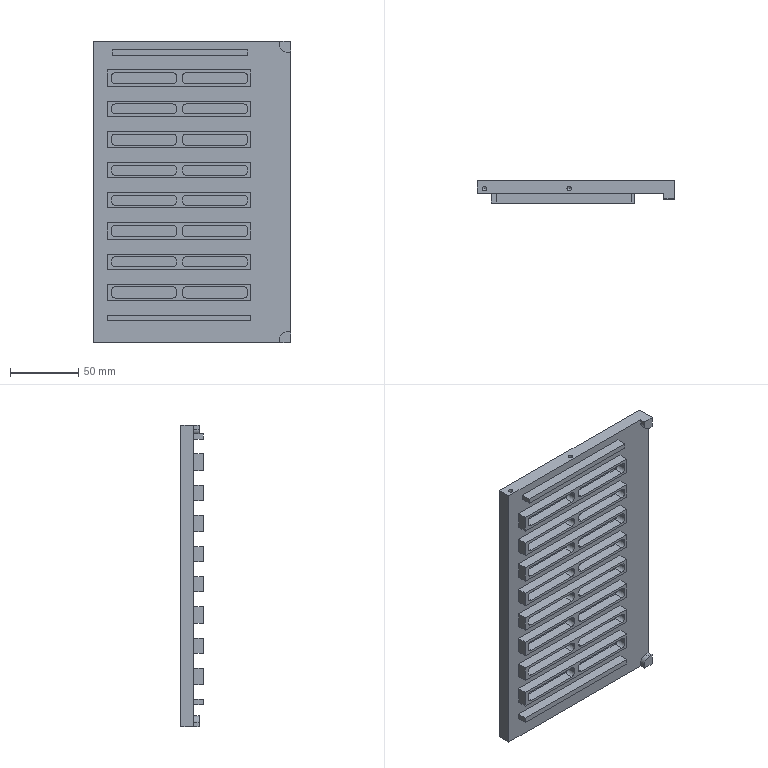NC program | NX | posted with a generic post | part box 144.5 x 16.5 x 221 mm
Lines 9456 to 11164 of 11164:
(PLANAR_MILL_4 , TOOL : D8-25-D8-60-3T-FINISH)
N18892 T04 M6
N18894 G54
N18896 G17 G0 G90 X-116.5 Y-64.45 B0. C0. S4200 M3
N18898 G43 Z20. H4
N18900 Z-1.1 B-180. C-180.
N18902 G94 G1 Z-3.1 F800.
N18904 X-110.5
N18906 X-102.5
N18908 X-96.5
N18910 Z-1.1
N18912 G0 Z20.
N18914 X-116.5 Y-69.25
N18916 Z-1.1
N18918 G1 Z-3.1
N18920 X-110.5
N18922 X-102.5
N18924 X-96.5
N18926 Z-1.1
N18928 G0 Z20.
N18930 X96.5 Y-64.45
N18932 Z-1.1
N18934 G1 Z-3.1
N18936 X102.5
N18938 X110.5
N18940 X116.5
N18942 Z-1.1
N18944 G0 Z20.
N18946 X96.5 Y-69.25
N18948 Z-1.1
N18950 G1 Z-3.1
N18952 X102.5
N18954 X110.5
N18956 X116.5
N18958 Z-1.1
N18960 G0 Z20.
(PLANAR_MILL_2_COPY_2 , TOOL : D8-25-D8-60-3T-FINISH)
N18962 X-112.5 Y78.25
N18964 Z-4.97
N18966 G1 Z-6.97 F1200.
N18968 Y74.25
N18970 G3 X-110.5 Y72.25 R2.
N18972 G1 X110.5
N18974 Y-60.2
N18976 X107.5
N18978 G3 X98.45 Y-69.25 R9.05
N18980 G1 Y-72.25
N18982 X-98.45
N18984 Y-69.25
N18986 G3 X-107.5 Y-60.2 R9.05
N18988 G1 X-110.5
N18990 Y72.25
N18992 X-104.9 Y66.65
N18994 X-99.614
N18996 X-92.5 Y67.84
N18998 X-99.614 Y66.65
N19000 G3 X-99.67 Y66.3 R1.12
N19002 G1 Y-46.8
N19004 G3 X-98.55 Y-47.92 R1.12
N19006 G1 X-86.45
N19008 G3 X-85.33 Y-46.8 R1.12
N19010 G1 Y66.3
N19012 G3 X-85.386 Y66.65 R1.12
N19014 G1 X-86.45 Y66.3
N19016 Y-46.8
N19018 X-98.55
N19020 Y66.3
N19022 X-86.45
N19024 X-85.386 Y66.65
N19026 X-84.814
N19028 X-80.889 Y67.42
N19030 X-66.311
N19032 G2 X-66.052 Y68.25 R4.
N19034 G1 X-81.148
N19036 G2 X-80.889 Y67.42 R4.
N19038 G1 X-84.814 Y66.65
N19040 G3 X-84.87 Y66.3 R1.12
N19042 G1 Y-46.8
N19044 G3 X-83.75 Y-47.92 R1.12
N19046 G1 X-63.45
N19048 G3 X-62.33 Y-46.8 R1.12
N19050 G1 Y66.3
N19052 G3 X-62.386 Y66.65 R1.12
N19054 G1 X-63.45 Y66.3
N19056 Y-46.8
N19058 X-83.75
N19060 Y66.3
N19062 X-63.45
N19064 X-62.386 Y66.65
N19066 X-61.814
N19068 X-57.889 Y67.42
N19070 X-44.311
N19072 G2 X-44.052 Y68.25 R4.
N19074 G1 X-58.148
N19076 G2 X-57.889 Y67.42 R4.
N19078 G1 X-61.814 Y66.65
N19080 G3 X-61.87 Y66.3 R1.12
N19082 G1 Y-46.8
N19084 G3 X-60.75 Y-47.92 R1.12
N19086 G1 X-41.45
N19088 G3 X-40.33 Y-46.8 R1.12
N19090 G1 Y66.3
N19092 G3 X-40.386 Y66.65 R1.12
N19094 G1 X-41.45 Y66.3
N19096 Y-46.8
N19098 X-60.75
N19100 Y66.3
N19102 X-41.45
N19104 X-40.386 Y66.65
N19106 X-39.814
N19108 X-35.889 Y67.42
N19110 X-21.311
N19112 G2 X-21.052 Y68.25 R4.
N19114 G1 X-36.148
N19116 G2 X-35.889 Y67.42 R4.
N19118 G1 X-39.814 Y66.65
N19120 G3 X-39.87 Y66.3 R1.12
N19122 G1 Y-46.8
N19124 G3 X-38.75 Y-47.92 R1.12
N19126 G1 X-18.45
N19128 G3 X-17.33 Y-46.8 R1.12
N19130 G1 Y66.3
N19132 G3 X-17.386 Y66.65 R1.12
N19134 G1 X-18.45 Y66.3
N19136 Y-46.8
N19138 X-38.75
N19140 Y66.3
N19142 X-18.45
N19144 X-17.386 Y66.65
N19146 X-16.814
N19148 X-12.889 Y67.42
N19150 X0.689
N19152 G2 X0.948 Y68.25 R4.
N19154 G1 X-13.148
N19156 G2 X-12.889 Y67.42 R4.
N19158 G1 X-16.814 Y66.65
N19160 G3 X-16.87 Y66.3 R1.12
N19162 G1 Y-46.8
N19164 G3 X-15.75 Y-47.92 R1.12
N19166 G1 X3.55
N19168 G3 X4.67 Y-46.8 R1.12
N19170 G1 Y66.3
N19172 G3 X4.614 Y66.65 R1.12
N19174 G1 X3.55 Y66.3
N19176 Y-46.8
N19178 X-15.75
N19180 Y66.3
N19182 X3.55
N19184 X4.614 Y66.65
N19186 X5.186
N19188 X9.111 Y67.42
N19190 X22.689
N19192 G2 X22.948 Y68.25 R4.
N19194 G1 X8.852
N19196 G2 X9.111 Y67.42 R4.
N19198 G1 X5.186 Y66.65
N19200 G3 X5.13 Y66.3 R1.12
N19202 G1 Y-46.8
N19204 G3 X6.25 Y-47.92 R1.12
N19206 G1 X25.55
N19208 G3 X26.67 Y-46.8 R1.12
N19210 G1 Y66.3
N19212 G3 X26.614 Y66.65 R1.12
N19214 G1 X25.55 Y66.3
N19216 Y-46.8
N19218 X6.25
N19220 Y66.3
N19222 X25.55
N19224 X26.614 Y66.65
N19226 X27.186
N19228 X31.111 Y67.42
N19230 X45.689
N19232 G2 X45.948 Y68.25 R4.
N19234 G1 X30.852
N19236 G2 X31.111 Y67.42 R4.
N19238 G1 X27.186 Y66.65
N19240 G3 X27.13 Y66.3 R1.12
N19242 G1 Y-46.8
N19244 G3 X28.25 Y-47.92 R1.12
N19246 G1 X48.55
N19248 G3 X49.67 Y-46.8 R1.12
N19250 G1 Y66.3
N19252 G3 X49.614 Y66.65 R1.12
N19254 G1 X48.55 Y66.3
N19256 Y-46.8
N19258 X28.25
N19260 Y66.3
N19262 X48.55
N19264 X49.614 Y66.65
N19266 X50.186
N19268 X54.111 Y67.42
N19270 X67.689
N19272 G2 X67.948 Y68.25 R4.
N19274 G1 X53.852
N19276 G2 X54.111 Y67.42 R4.
N19278 G1 X50.186 Y66.65
N19280 G3 X50.13 Y66.3 R1.12
N19282 G1 Y-46.8
N19284 G3 X51.25 Y-47.92 R1.12
N19286 G1 X70.55
N19288 G3 X71.67 Y-46.8 R1.12
N19290 G1 Y66.3
N19292 G3 X71.614 Y66.65 R1.12
N19294 G1 X70.55 Y66.3
N19296 Y-46.8
N19298 X51.25
N19300 Y66.3
N19302 X70.55
N19304 X71.614 Y66.65
N19306 X72.186
N19308 X76.111 Y67.42
N19310 X90.689
N19312 G2 X90.948 Y68.25 R4.
N19314 G1 X75.852
N19316 G2 X76.111 Y67.42 R4.
N19318 G1 X72.186 Y66.65
N19320 G3 X72.13 Y66.3 R1.12
N19322 G1 Y-46.8
N19324 G3 X73.25 Y-47.92 R1.12
N19326 G1 X93.55
N19328 G3 X94.67 Y-46.8 R1.12
N19330 G1 Y66.3
N19332 G3 X94.614 Y66.65 R1.12
N19334 G1 X93.55 Y66.3
N19336 Y-46.8
N19338 X73.25
N19340 Y66.3
N19342 X93.55
N19344 X94.614 Y66.65
N19346 X104.9
N19348 Y63.42
N19350 X96.25
N19352 G3 X95.13 Y62.3 R1.12
N19354 G1 Y-44.8
N19356 G3 X96.25 Y-45.92 R1.12
N19358 G1 X104.9
N19360 Y-44.8
N19362 X96.25
N19364 Y62.3
N19366 X108.15
N19368 Y-44.8
N19370 X104.9
N19372 Y-45.92
N19374 Y-54.833
N19376 G3 X93.083 Y-66.65 R14.65
N19378 G1 X-93.083
N19380 G3 X-98.274 Y-57.87 R14.65
N19382 G1 X-94.747 Y-53.52
N19384 X-86.45
N19386 G3 X-85.1 Y-53.383 R6.72
N19388 X-83.75 Y-53.52 R6.72
N19390 G1 X-63.45
N19392 G3 X-62.1 Y-53.383 R6.72
N19394 X-60.75 Y-53.52 R6.72
N19396 G1 X-41.45
N19398 G3 X-40.1 Y-53.383 R6.72
N19400 X-38.75 Y-53.52 R6.72
N19402 G1 X-18.45
N19404 G3 X-17.1 Y-53.383 R6.72
N19406 X-15.75 Y-53.52 R6.72
N19408 G1 X3.55
N19410 G3 X4.9 Y-53.383 R6.72
N19412 X6.25 Y-53.52 R6.72
N19414 G1 X25.55
N19416 G3 X26.9 Y-53.383 R6.72
N19418 X28.25 Y-53.52 R6.72
N19420 G1 X48.55
N19422 G3 X49.9 Y-53.383 R6.72
N19424 X51.25 Y-53.52 R6.72
N19426 G1 X70.55
N19428 G3 X71.9 Y-53.383 R6.72
N19430 X73.25 Y-53.52 R6.72
N19432 G1 X93.55
N19434 G3 X94.925 Y-53.378 R6.72
N19436 G1 X99.428 Y-50.99
N19438 X94.925 Y-53.378
N19440 G3 X88.985 Y-61.05 R20.25
N19442 G1 X-88.985
N19444 G3 X-94.747 Y-53.52 R20.25
N19446 G1 X-99.565 Y-52.064
N19448 X-94.747 Y-53.52
N19450 X-86.965 Y-57.12
N19452 X-86.45
N19454 G3 X-85.1 Y-57.031 R10.32
N19456 X-83.75 Y-57.12 R10.32
N19458 G1 X-63.45
N19460 G3 X-62.1 Y-57.031 R10.32
N19462 X-60.75 Y-57.12 R10.32
N19464 G1 X-41.45
N19466 G3 X-40.1 Y-57.031 R10.32
N19468 X-38.75 Y-57.12 R10.32
N19470 G1 X-18.45
N19472 G3 X-17.1 Y-57.031 R10.32
N19474 X-15.75 Y-57.12 R10.32
N19476 G1 X3.55
N19478 G3 X4.9 Y-57.031 R10.32
N19480 X6.25 Y-57.12 R10.32
N19482 G1 X25.55
N19484 G3 X26.9 Y-57.031 R10.32
N19486 X28.25 Y-57.12 R10.32
N19488 G1 X48.55
N19490 G3 X49.9 Y-57.031 R10.32
N19492 X51.25 Y-57.12 R10.32
N19494 G1 X70.55
N19496 G3 X71.9 Y-57.031 R10.32
N19498 X73.25 Y-57.12 R10.32
N19500 G1 X86.965
N19502 G3 X86.774 Y-57.45 R23.85
N19504 G1 X-86.774
N19506 G3 X-86.965 Y-57.12 R23.85
N19508 G1 X-94.747 Y-53.52
N19510 X-98.274 Y-57.87
N19512 G3 X-104.9 Y-54.833 R14.65
N19514 G1 Y66.65
N19516 G3 X-106.9 Y68.65 R2.
N19518 G1 Y78.25
N19520 Z-4.97
N19522 G0 Z20.
(PLANAR_MILL_2 , TOOL : D8-25-D8-60-3T-FINISH)
N19524 X-85.73 Y68.28
N19526 Z-4.94
N19528 G1 Z-6.94
N19530 G3 X-83.73 Y66.28 R2.
N19532 G1 X-63.47
N19534 Y-46.78
N19536 X-83.73
N19538 Y66.28
N19540 G3 X-85.73 Y68.28 R2.
N19542 G1 X-84.47
N19544 G3 X-86.47 Y66.28 R2.
N19546 G1 Y-46.78
N19548 X-98.53
N19550 Y66.28
N19552 X-86.47
N19554 G3 X-84.47 Y68.28 R2.
N19556 G1 Z-4.94
N19558 G0 Z20.
N19560 X-62.73
N19562 Z-4.94
N19564 G1 Z-6.94
N19566 G3 X-60.73 Y66.28 R2.
N19568 G1 X-41.47
N19570 Y-46.78
N19572 X-60.73
N19574 Y66.28
N19576 G3 X-62.73 Y68.28 R2.
N19578 G1 Z-4.94
N19580 G0 Z20.
N19582 X-40.73
N19584 Z-4.94
N19586 G1 Z-6.94
N19588 G3 X-38.73 Y66.28 R2.
N19590 G1 X-18.47
N19592 Y-46.78
N19594 X-38.73
N19596 Y66.28
N19598 G3 X-40.73 Y68.28 R2.
N19600 G1 Z-4.94
N19602 G0 Z20.
N19604 X-17.73
N19606 Z-4.94
N19608 G1 Z-6.94
N19610 G3 X-15.73 Y66.28 R2.
N19612 G1 X3.53
N19614 Y-46.78
N19616 X-15.73
N19618 Y66.28
N19620 G3 X-17.73 Y68.28 R2.
N19622 G1 Z-4.94
N19624 G0 Z20.
N19626 X4.27
N19628 Z-4.94
N19630 G1 Z-6.94
N19632 G3 X6.27 Y66.28 R2.
N19634 G1 X25.53
N19636 Y-46.78
N19638 X6.27
N19640 Y66.28
N19642 G3 X4.27 Y68.28 R2.
N19644 G1 Z-4.94
N19646 G0 Z20.
N19648 X26.27
N19650 Z-4.94
N19652 G1 Z-6.94
N19654 G3 X28.27 Y66.28 R2.
N19656 G1 X48.53
N19658 Y-46.78
N19660 X28.27
N19662 Y66.28
N19664 G3 X26.27 Y68.28 R2.
N19666 G1 Z-4.94
N19668 G0 Z20.
N19670 X49.27
N19672 Z-4.94
N19674 G1 Z-6.94
N19676 G3 X51.27 Y66.28 R2.
N19678 G1 X70.53
N19680 Y-46.78
N19682 X51.27
N19684 Y66.28
N19686 G3 X49.27 Y68.28 R2.
N19688 G1 Z-4.94
N19690 G0 Z20.
N19692 X95.53
N19694 Z-4.94
N19696 G1 Z-6.94
N19698 G3 X93.53 Y66.28 R2.
N19700 G1 Y-46.78
N19702 X73.27
N19704 Y66.28
N19706 X93.53
N19708 G3 X95.53 Y68.28 R2.
N19710 G1 X94.27 Y64.28
N19712 G3 X96.27 Y62.28 R2.
N19714 G1 X108.13
N19716 Y-44.78
N19718 X96.27
N19720 Y62.28
N19722 G3 X95.27 Y63.28 R1.
N19724 G1 X95.53 Y64.138
N19726 Z-4.94
N19728 G0 Z20.
(PLANAR_MILL_2_COPY_2_COPY , TOOL : D8-25-D8-60-3T-FINISH)
N19730 X-112.5 Y78.25
N19732 Z-5.
N19734 G1 Z-7. F800.
N19736 Y74.25
N19738 G3 X-110.5 Y72.25 R2.
N19740 G1 X110.5
N19742 Y-60.2
N19744 X107.5
N19746 G3 X98.45 Y-69.25 R9.05
N19748 G1 Y-72.25
N19750 X-98.45
N19752 Y-69.25
N19754 G3 X-107.5 Y-60.2 R9.05
N19756 G1 X-110.5
N19758 Y72.25
N19760 X-104.9 Y66.65
N19762 X-99.614
N19764 X-92.5 Y67.84
N19766 X-99.614 Y66.65
N19768 G3 X-99.67 Y66.3 R1.12
N19770 G1 Y-46.8
N19772 G3 X-98.55 Y-47.92 R1.12
N19774 G1 X-86.45
N19776 G3 X-85.33 Y-46.8 R1.12
N19778 G1 Y66.3
N19780 G3 X-85.386 Y66.65 R1.12
N19782 G1 X-86.45 Y66.3
N19784 Y-46.8
N19786 X-98.55
N19788 Y66.3
N19790 X-86.45
N19792 X-85.386 Y66.65
N19794 X-84.814
N19796 X-80.889 Y67.42
N19798 X-66.311
N19800 G2 X-66.052 Y68.25 R4.
N19802 G1 X-81.148
N19804 G2 X-80.889 Y67.42 R4.
N19806 G1 X-84.814 Y66.65
N19808 G3 X-84.87 Y66.3 R1.12
N19810 G1 Y-46.8
N19812 G3 X-83.75 Y-47.92 R1.12
N19814 G1 X-63.45
N19816 G3 X-62.33 Y-46.8 R1.12
N19818 G1 Y66.3
N19820 G3 X-62.386 Y66.65 R1.12
N19822 G1 X-63.45 Y66.3
N19824 Y-46.8
N19826 X-83.75
N19828 Y66.3
N19830 X-63.45
N19832 X-62.386 Y66.65
N19834 X-61.814
N19836 X-57.889 Y67.42
N19838 X-44.311
N19840 G2 X-44.052 Y68.25 R4.
N19842 G1 X-58.148
N19844 G2 X-57.889 Y67.42 R4.
N19846 G1 X-61.814 Y66.65
N19848 G3 X-61.87 Y66.3 R1.12
N19850 G1 Y-46.8
N19852 G3 X-60.75 Y-47.92 R1.12
N19854 G1 X-41.45
N19856 G3 X-40.33 Y-46.8 R1.12
N19858 G1 Y66.3
N19860 G3 X-40.386 Y66.65 R1.12
N19862 G1 X-41.45 Y66.3
N19864 Y-46.8
N19866 X-60.75
N19868 Y66.3
N19870 X-41.45
N19872 X-40.386 Y66.65
N19874 X-39.814
N19876 X-35.889 Y67.42
N19878 X-21.311
N19880 G2 X-21.052 Y68.25 R4.
N19882 G1 X-36.148
N19884 G2 X-35.889 Y67.42 R4.
N19886 G1 X-39.814 Y66.65
N19888 G3 X-39.87 Y66.3 R1.12
N19890 G1 Y-46.8
N19892 G3 X-38.75 Y-47.92 R1.12
N19894 G1 X-18.45
N19896 G3 X-17.33 Y-46.8 R1.12
N19898 G1 Y66.3
N19900 G3 X-17.386 Y66.65 R1.12
N19902 G1 X-18.45 Y66.3
N19904 Y-46.8
N19906 X-38.75
N19908 Y66.3
N19910 X-18.45
N19912 X-17.386 Y66.65
N19914 X-16.814
N19916 X-12.889 Y67.42
N19918 X0.689
N19920 G2 X0.948 Y68.25 R4.
N19922 G1 X-13.148
N19924 G2 X-12.889 Y67.42 R4.
N19926 G1 X-16.814 Y66.65
N19928 G3 X-16.87 Y66.3 R1.12
N19930 G1 Y-46.8
N19932 G3 X-15.75 Y-47.92 R1.12
N19934 G1 X3.55
N19936 G3 X4.67 Y-46.8 R1.12
N19938 G1 Y66.3
N19940 G3 X4.614 Y66.65 R1.12
N19942 G1 X3.55 Y66.3
N19944 Y-46.8
N19946 X-15.75
N19948 Y66.3
N19950 X3.55
N19952 X4.614 Y66.65
N19954 X5.186
N19956 X9.111 Y67.42
N19958 X22.689
N19960 G2 X22.948 Y68.25 R4.
N19962 G1 X8.852
N19964 G2 X9.111 Y67.42 R4.
N19966 G1 X5.186 Y66.65
N19968 G3 X5.13 Y66.3 R1.12
N19970 G1 Y-46.8
N19972 G3 X6.25 Y-47.92 R1.12
N19974 G1 X25.55
N19976 G3 X26.67 Y-46.8 R1.12
N19978 G1 Y66.3
N19980 G3 X26.614 Y66.65 R1.12
N19982 G1 X25.55 Y66.3
N19984 Y-46.8
N19986 X6.25
N19988 Y66.3
N19990 X25.55
N19992 X26.614 Y66.65
N19994 X27.186
N19996 X31.111 Y67.42
N19998 X45.689
N20000 G2 X45.948 Y68.25 R4.
N20002 G1 X30.852
N20004 G2 X31.111 Y67.42 R4.
N20006 G1 X27.186 Y66.65
N20008 G3 X27.13 Y66.3 R1.12
N20010 G1 Y-46.8
N20012 G3 X28.25 Y-47.92 R1.12
N20014 G1 X48.55
N20016 G3 X49.67 Y-46.8 R1.12
N20018 G1 Y66.3
N20020 G3 X49.614 Y66.65 R1.12
N20022 G1 X48.55 Y66.3
N20024 Y-46.8
N20026 X28.25
N20028 Y66.3
N20030 X48.55
N20032 X49.614 Y66.65
N20034 X50.186
N20036 X54.111 Y67.42
N20038 X67.689
N20040 G2 X67.948 Y68.25 R4.
N20042 G1 X53.852
N20044 G2 X54.111 Y67.42 R4.
N20046 G1 X50.186 Y66.65
N20048 G3 X50.13 Y66.3 R1.12
N20050 G1 Y-46.8
N20052 G3 X51.25 Y-47.92 R1.12
N20054 G1 X70.55
N20056 G3 X71.67 Y-46.8 R1.12
N20058 G1 Y66.3
N20060 G3 X71.614 Y66.65 R1.12
N20062 G1 X70.55 Y66.3
N20064 Y-46.8
N20066 X51.25
N20068 Y66.3
N20070 X70.55
N20072 X71.614 Y66.65
N20074 X72.186
N20076 X76.111 Y67.42
N20078 X90.689
N20080 G2 X90.948 Y68.25 R4.
N20082 G1 X75.852
N20084 G2 X76.111 Y67.42 R4.
N20086 G1 X72.186 Y66.65
N20088 G3 X72.13 Y66.3 R1.12
N20090 G1 Y-46.8
N20092 G3 X73.25 Y-47.92 R1.12
N20094 G1 X93.55
N20096 G3 X94.67 Y-46.8 R1.12
N20098 G1 Y66.3
N20100 G3 X94.614 Y66.65 R1.12
N20102 G1 X93.55 Y66.3
N20104 Y-46.8
N20106 X73.25
N20108 Y66.3
N20110 X93.55
N20112 X94.614 Y66.65
N20114 X104.9
N20116 Y63.42
N20118 X96.25
N20120 G3 X95.13 Y62.3 R1.12
N20122 G1 Y-44.8
N20124 G3 X96.25 Y-45.92 R1.12
N20126 G1 X104.9
N20128 Y-44.8
N20130 X96.25
N20132 Y62.3
N20134 X108.15
N20136 Y-44.8
N20138 X104.9
N20140 Y-45.92
N20142 Y-54.833
N20144 G3 X93.083 Y-66.65 R14.65
N20146 G1 X-93.083
N20148 G3 X-98.274 Y-57.87 R14.65
N20150 G1 X-94.747 Y-53.52
N20152 X-86.45
N20154 G3 X-85.1 Y-53.383 R6.72
N20156 X-83.75 Y-53.52 R6.72
N20158 G1 X-63.45
N20160 G3 X-62.1 Y-53.383 R6.72
N20162 X-60.75 Y-53.52 R6.72
N20164 G1 X-41.45
N20166 G3 X-40.1 Y-53.383 R6.72
N20168 X-38.75 Y-53.52 R6.72
N20170 G1 X-18.45
N20172 G3 X-17.1 Y-53.383 R6.72
N20174 X-15.75 Y-53.52 R6.72
N20176 G1 X3.55
N20178 G3 X4.9 Y-53.383 R6.72
N20180 X6.25 Y-53.52 R6.72
N20182 G1 X25.55
N20184 G3 X26.9 Y-53.383 R6.72
N20186 X28.25 Y-53.52 R6.72
N20188 G1 X48.55
N20190 G3 X49.9 Y-53.383 R6.72
N20192 X51.25 Y-53.52 R6.72
N20194 G1 X70.55
N20196 G3 X71.9 Y-53.383 R6.72
N20198 X73.25 Y-53.52 R6.72
N20200 G1 X93.55
N20202 G3 X94.925 Y-53.378 R6.72
N20204 G1 X99.428 Y-50.99
N20206 X94.925 Y-53.378
N20208 G3 X88.985 Y-61.05 R20.25
N20210 G1 X-88.985
N20212 G3 X-94.747 Y-53.52 R20.25
N20214 G1 X-99.565 Y-52.064
N20216 X-94.747 Y-53.52
N20218 X-86.965 Y-57.12
N20220 X-86.45
N20222 G3 X-85.1 Y-57.031 R10.32
N20224 X-83.75 Y-57.12 R10.32
N20226 G1 X-63.45
N20228 G3 X-62.1 Y-57.031 R10.32
N20230 X-60.75 Y-57.12 R10.32
N20232 G1 X-41.45
N20234 G3 X-40.1 Y-57.031 R10.32
N20236 X-38.75 Y-57.12 R10.32
N20238 G1 X-18.45
N20240 G3 X-17.1 Y-57.031 R10.32
N20242 X-15.75 Y-57.12 R10.32
N20244 G1 X3.55
N20246 G3 X4.9 Y-57.031 R10.32
N20248 X6.25 Y-57.12 R10.32
N20250 G1 X25.55
N20252 G3 X26.9 Y-57.031 R10.32
N20254 X28.25 Y-57.12 R10.32
N20256 G1 X48.55
N20258 G3 X49.9 Y-57.031 R10.32
N20260 X51.25 Y-57.12 R10.32
N20262 G1 X70.55
N20264 G3 X71.9 Y-57.031 R10.32
N20266 X73.25 Y-57.12 R10.32
N20268 G1 X86.965
N20270 G3 X86.774 Y-57.45 R23.85
N20272 G1 X-86.774
N20274 G3 X-86.965 Y-57.12 R23.85
N20276 G1 X-94.747 Y-53.52
N20278 X-98.274 Y-57.87
N20280 G3 X-104.9 Y-54.833 R14.65
N20282 G1 Y66.65
N20284 G3 X-106.9 Y68.65 R2.
N20286 G1 Y78.25
N20288 Z-5.
N20290 G0 Z20.
(PLANAR_MILL_2_COPY_3 , TOOL : D8-25-D8-60-3T-FINISH)
N20292 X-85.7 Y68.25
N20294 Z-4.98
N20296 G1 Z-6.98
N20298 G3 X-83.7 Y66.25 R2.
N20300 G1 X-63.5
N20302 Y-46.75
N20304 X-83.7
N20306 Y66.25
N20308 G3 X-85.7 Y68.25 R2.
N20310 G1 X-84.5
N20312 G3 X-86.5 Y66.25 R2.
N20314 G1 Y-46.75
N20316 X-98.5
N20318 Y66.25
N20320 X-86.5
N20322 G3 X-84.5 Y68.25 R2.
N20324 G1 Z-4.98
N20326 G0 Z20.
N20328 X-62.7
N20330 Z-4.98
N20332 G1 Z-6.98
N20334 G3 X-60.7 Y66.25 R2.
N20336 G1 X-41.5
N20338 Y-46.75
N20340 X-60.7
N20342 Y66.25
N20344 G3 X-62.7 Y68.25 R2.
N20346 G1 Z-4.98
N20348 G0 Z20.
N20350 X-40.7
N20352 Z-4.98
N20354 G1 Z-6.98
N20356 G3 X-38.7 Y66.25 R2.
N20358 G1 X-18.5
N20360 Y-46.75
N20362 X-38.7
N20364 Y66.25
N20366 G3 X-40.7 Y68.25 R2.
N20368 G1 Z-4.98
N20370 G0 Z20.
N20372 X-17.7
N20374 Z-4.98
N20376 G1 Z-6.98
N20378 G3 X-15.7 Y66.25 R2.
N20380 G1 X3.5
N20382 Y-46.75
N20384 X-15.7
N20386 Y66.25
N20388 G3 X-17.7 Y68.25 R2.
N20390 G1 Z-4.98
N20392 G0 Z20.
N20394 X4.3
N20396 Z-4.98
N20398 G1 Z-6.98
N20400 G3 X6.3 Y66.25 R2.
N20402 G1 X25.5
N20404 Y-46.75
N20406 X6.3
N20408 Y66.25
N20410 G3 X4.3 Y68.25 R2.
N20412 G1 Z-4.98
N20414 G0 Z20.
N20416 X26.3
N20418 Z-4.98
N20420 G1 Z-6.98
N20422 G3 X28.3 Y66.25 R2.
N20424 G1 X48.5
N20426 Y-46.75
N20428 X28.3
N20430 Y66.25
N20432 G3 X26.3 Y68.25 R2.
N20434 G1 Z-4.98
N20436 G0 Z20.
N20438 X49.3
N20440 Z-4.98
N20442 G1 Z-6.98
N20444 G3 X51.3 Y66.25 R2.
N20446 G1 X70.5
N20448 Y-46.75
N20450 X51.3
N20452 Y66.25
N20454 G3 X49.3 Y68.25 R2.
N20456 G1 Z-4.98
N20458 G0 Z20.
N20460 X95.5
N20462 Z-4.98
N20464 G1 Z-6.98
N20466 G3 X93.5 Y66.25 R2.
N20468 G1 Y-46.75
N20470 X73.3
N20472 Y66.25
N20474 X93.5
N20476 G3 X95.5 Y68.25 R2.
N20478 G1 X94.3 Y64.25
N20480 G3 X96.3 Y62.25 R2.
N20482 G1 X108.1
N20484 Y-44.75
N20486 X96.3
N20488 Y62.25
N20490 G3 X95.3 Y63.25 R1.
N20492 G1 X95.5 Y64.083
N20494 Z-4.98
N20496 G0 Z20.
(PLANAR_MILL_2_COPY , TOOL : D8-25-D8-60-3T-FINISH)
N20498 X-112.5 Y-58.25
N20500 Z-4.98
N20502 G1 Z-6.98
N20504 G3 X-110.5 Y-60.25 R2.
N20506 G1 X-107.5
N20508 G2 X-98.5 Y-69.25 R9.
N20510 G1 Y-72.25
N20512 G3 X-96.5 Y-74.25 R2.
N20514 G1 Z-4.98
N20516 G0 Z20.
N20518 X96.5
N20520 Z-4.98
N20522 G1 Z-6.98
N20524 G3 X98.5 Y-72.25 R2.
N20526 G1 Y-69.25
N20528 G2 X107.5 Y-60.25 R9.
N20530 G1 X110.5
N20532 G3 X112.5 Y-58.25 R2.
N20534 G1 Z-4.98
N20536 G0 Z20.
N20538 M5
(PLANAR_MILL_3 , TOOL : D5-15-D6-50-3T-FINISH)
N20540 T05 M6
N20542 G54
N20544 G17 G0 G90 X-75.18 Y46.68 B0. C0. S4200 M3
N20546 G43 Z20. H5
N20548 Z-6. B-180. C-180.
N20550 G94 G1 Y35.25 Z-7. F800.
N20552 Y14.25
N20554 G3 X-74.7 Y13.77 R0.48
N20556 G1 X-72.5
N20558 G3 X-72.02 Y14.25 R0.48
N20560 G1 Y56.25
N20562 G3 X-72.5 Y56.73 R0.48
N20564 G1 X-74.7
N20566 G3 X-75.18 Y56.25 R0.48
N20568 G1 Y35.25
N20570 Z-6.
N20572 G0 Z20.
N20574 X-52.18 Y46.68
N20576 Z-6.
N20578 G1 Y35.25 Z-7.
N20580 Y14.25
N20582 G3 X-51.7 Y13.77 R0.48
N20584 G1 X-50.5
N20586 G3 X-50.02 Y14.25 R0.48
N20588 G1 Y56.25
N20590 G3 X-50.5 Y56.73 R0.48
N20592 G1 X-51.7
N20594 G3 X-52.18 Y56.25 R0.48
N20596 G1 Y35.25
N20598 Z-6.
N20600 G0 Z20.
N20602 X-30.18 Y46.68
N20604 Z-6.
N20606 G1 Y35.25 Z-7.
N20608 Y14.25
N20610 G3 X-29.7 Y13.77 R0.48
N20612 G1 X-27.5
N20614 G3 X-27.02 Y14.25 R0.48
N20616 G1 Y56.25
N20618 G3 X-27.5 Y56.73 R0.48
N20620 G1 X-29.7
N20622 G3 X-30.18 Y56.25 R0.48
N20624 G1 Y35.25
N20626 Z-6.
N20628 G0 Z20.
N20630 X-7.18 Y46.68
N20632 Z-6.
N20634 G1 Y35.25 Z-7.
N20636 Y14.25
N20638 G3 X-6.7 Y13.77 R0.48
N20640 G1 X-5.5
N20642 G3 X-5.02 Y14.25 R0.48
N20644 G1 Y56.25
N20646 G3 X-5.5 Y56.73 R0.48
N20648 G1 X-6.7
N20650 G3 X-7.18 Y56.25 R0.48
N20652 G1 Y35.25
N20654 Z-6.
N20656 G0 Z20.
N20658 X14.82 Y46.68
N20660 Z-6.
N20662 G1 Y35.25 Z-7.
N20664 Y14.25
N20666 G3 X15.3 Y13.77 R0.48
N20668 G1 X16.5
N20670 G3 X16.98 Y14.25 R0.48
N20672 G1 Y56.25
N20674 G3 X16.5 Y56.73 R0.48
N20676 G1 X15.3
N20678 G3 X14.82 Y56.25 R0.48
N20680 G1 Y35.25
N20682 Z-6.
N20684 G0 Z20.
N20686 X36.82 Y46.68
N20688 Z-6.
N20690 G1 Y35.25 Z-7.
N20692 Y14.25
N20694 G3 X37.3 Y13.77 R0.48
N20696 G1 X39.5
N20698 G3 X39.98 Y14.25 R0.48
N20700 G1 Y56.25
N20702 G3 X39.5 Y56.73 R0.48
N20704 G1 X37.3
N20706 G3 X36.82 Y56.25 R0.48
N20708 G1 Y35.25
N20710 Z-6.
N20712 G0 Z20.
N20714 X59.82 Y46.68
N20716 Z-6.
N20718 G1 Y35.25 Z-7.
N20720 Y14.25
N20722 G3 X60.3 Y13.77 R0.48
N20724 G1 X61.5
N20726 G3 X61.98 Y14.25 R0.48
N20728 G1 Y56.25
N20730 G3 X61.5 Y56.73 R0.48
N20732 G1 X60.3
N20734 G3 X59.82 Y56.25 R0.48
N20736 G1 Y35.25
N20738 Z-6.
N20740 G0 Z20.
N20742 X84.98 Y23.82
N20744 Z-6.
N20746 G1 Y35.25 Z-7.
N20748 Y56.25
N20750 G3 X84.5 Y56.73 R0.48
N20752 G1 X82.3
N20754 G3 X81.82 Y56.25 R0.48
N20756 G1 Y14.25
N20758 G3 X82.3 Y13.77 R0.48
N20760 G1 X84.5
N20762 G3 X84.98 Y14.25 R0.48
N20764 G1 Y35.25
N20766 Z-6.
N20768 G0 Z20.
N20770 Y-28.18
N20772 Z-6.
N20774 G1 Y-16.75 Z-7.
N20776 Y4.25
N20778 G3 X84.5 Y4.73 R0.48
N20780 G1 X82.3
N20782 G3 X81.82 Y4.25 R0.48
N20784 G1 Y-37.75
N20786 G3 X82.3 Y-38.23 R0.48
N20788 G1 X84.5
N20790 G3 X84.98 Y-37.75 R0.48
N20792 G1 Y-16.75
N20794 Z-6.
N20796 G0 Z20.
N20798 X61.98 Y-28.18
N20800 Z-6.
N20802 G1 Y-16.75 Z-7.
N20804 Y4.25
N20806 G3 X61.5 Y4.73 R0.48
N20808 G1 X60.3
N20810 G3 X59.82 Y4.25 R0.48
N20812 G1 Y-37.75
N20814 G3 X60.3 Y-38.23 R0.48
N20816 G1 X61.5
N20818 G3 X61.98 Y-37.75 R0.48
N20820 G1 Y-16.75
N20822 Z-6.
N20824 G0 Z20.
N20826 X39.98 Y-28.18
N20828 Z-6.
N20830 G1 Y-16.75 Z-7.
N20832 Y4.25
N20834 G3 X39.5 Y4.73 R0.48
N20836 G1 X37.3
N20838 G3 X36.82 Y4.25 R0.48
N20840 G1 Y-37.75
N20842 G3 X37.3 Y-38.23 R0.48
N20844 G1 X39.5
N20846 G3 X39.98 Y-37.75 R0.48
N20848 G1 Y-16.75
N20850 Z-6.
N20852 G0 Z20.
N20854 X16.98 Y-28.18
N20856 Z-6.
N20858 G1 Y-16.75 Z-7.
N20860 Y4.25
N20862 G3 X16.5 Y4.73 R0.48
N20864 G1 X15.3
N20866 G3 X14.82 Y4.25 R0.48
N20868 G1 Y-37.75
N20870 G3 X15.3 Y-38.23 R0.48
N20872 G1 X16.5
N20874 G3 X16.98 Y-37.75 R0.48
N20876 G1 Y-16.75
N20878 Z-6.
N20880 G0 Z20.
N20882 X-5.02 Y-28.18
N20884 Z-6.
N20886 G1 Y-16.75 Z-7.
N20888 Y4.25
N20890 G3 X-5.5 Y4.73 R0.48
N20892 G1 X-6.7
N20894 G3 X-7.18 Y4.25 R0.48
N20896 G1 Y-37.75
N20898 G3 X-6.7 Y-38.23 R0.48
N20900 G1 X-5.5
N20902 G3 X-5.02 Y-37.75 R0.48
N20904 G1 Y-16.75
N20906 Z-6.
N20908 G0 Z20.
N20910 X-27.02 Y-28.18
N20912 Z-6.
N20914 G1 Y-16.75 Z-7.
N20916 Y4.25
N20918 G3 X-27.5 Y4.73 R0.48
N20920 G1 X-29.7
N20922 G3 X-30.18 Y4.25 R0.48
N20924 G1 Y-37.75
N20926 G3 X-29.7 Y-38.23 R0.48
N20928 G1 X-27.5
N20930 G3 X-27.02 Y-37.75 R0.48
N20932 G1 Y-16.75
N20934 Z-6.
N20936 G0 Z20.
N20938 X-50.02 Y-28.18
N20940 Z-6.
N20942 G1 Y-16.75 Z-7.
N20944 Y4.25
N20946 G3 X-50.5 Y4.73 R0.48
N20948 G1 X-51.7
N20950 G3 X-52.18 Y4.25 R0.48
N20952 G1 Y-37.75
N20954 G3 X-51.7 Y-38.23 R0.48
N20956 G1 X-50.5
N20958 G3 X-50.02 Y-37.75 R0.48
N20960 G1 Y-16.75
N20962 Z-6.
N20964 G0 Z20.
N20966 X-75.18 Y-5.32
N20968 Z-6.
N20970 G1 Y-16.75 Z-7.
N20972 Y-37.75
N20974 G3 X-74.7 Y-38.23 R0.48
N20976 G1 X-72.5
N20978 G3 X-72.02 Y-37.75 R0.48
N20980 G1 Y4.25
N20982 G3 X-72.5 Y4.73 R0.48
N20984 G1 X-74.7
N20986 G3 X-75.18 Y4.25 R0.48
N20988 G1 Y-16.75
N20990 Z-6.
N20992 G0 Z20.
(PLANAR_MILL_3_COPY , TOOL : D5-15-D6-50-3T-FINISH)
N20994 X82.76 Y55.79
N20996 Z-4.98
N20998 G1 Z-6.98
N21000 X82.26 Y56.75
N21002 G3 X81.76 Y56.25 R0.5
N21004 G1 Y14.25
N21006 G3 X82.3 Y13.71 R0.54
N21008 G1 X84.5
N21010 G3 X85.04 Y14.25 R0.54
N21012 G1 Y56.25
N21014 G3 X84.5 Y56.79 R0.54
N21016 G1 X82.3
N21018 G3 X81.76 Y56.25 R0.54
N21020 X82.76 Y55.25 R1.
N21022 G1 Z-4.98
N21024 G0 Z20.
N21026 X60.76 Y15.25
N21028 Z-4.98
N21030 G1 Z-6.98
N21032 G3 X59.76 Y14.25 R1.
N21034 X60.3 Y13.71 R0.54
N21036 G1 X61.5
N21038 G3 X62.04 Y14.25 R0.54
N21040 G1 Y56.25
N21042 G3 X61.5 Y56.79 R0.54
N21044 G1 X60.3
N21046 G3 X59.76 Y56.25 R0.54
N21048 G1 Y14.25
N21050 G3 X60.26 Y13.75 R0.5
N21052 G1 X60.76 Y14.71
N21054 Z-4.98
N21056 G0 Z20.
N21058 X37.76 Y15.25
N21060 Z-4.98
N21062 G1 Z-6.98
N21064 G3 X36.76 Y14.25 R1.
N21066 X37.3 Y13.71 R0.54
N21068 G1 X39.5
N21070 G3 X40.04 Y14.25 R0.54
N21072 G1 Y56.25
N21074 G3 X39.5 Y56.79 R0.54
N21076 G1 X37.3
N21078 G3 X36.76 Y56.25 R0.54
N21080 G1 Y14.25
N21082 G3 X37.26 Y13.75 R0.5
N21084 G1 X37.76 Y14.71
N21086 Z-4.98
N21088 G0 Z20.
N21090 X15.76 Y15.25
N21092 Z-4.98
N21094 G1 Z-6.98
N21096 G3 X14.76 Y14.25 R1.
N21098 X15.3 Y13.71 R0.54
N21100 G1 X16.5
N21102 G3 X17.04 Y14.25 R0.54
N21104 G1 Y56.25
N21106 G3 X16.5 Y56.79 R0.54
N21108 G1 X15.3
N21110 G3 X14.76 Y56.25 R0.54
N21112 G1 Y14.25
N21114 G3 X15.26 Y13.75 R0.5
N21116 G1 X15.76 Y14.71
N21118 Z-4.98
N21120 G0 Z20.
N21122 X-6.24 Y15.25
N21124 Z-4.98
N21126 G1 Z-6.98
N21128 G3 X-7.24 Y14.25 R1.
N21130 X-6.7 Y13.71 R0.54
N21132 G1 X-5.5
N21134 G3 X-4.96 Y14.25 R0.54
N21136 G1 Y56.25
N21138 G3 X-5.5 Y56.79 R0.54
N21140 G1 X-6.7
N21142 G3 X-7.24 Y56.25 R0.54
N21144 G1 Y14.25
N21146 G3 X-6.74 Y13.75 R0.5
N21148 G1 X-6.24 Y14.71
N21150 Z-4.98
N21152 G0 Z20.
N21154 X-29.24 Y15.25
N21156 Z-4.98
N21158 G1 Z-6.98
N21160 G3 X-30.24 Y14.25 R1.
N21162 X-29.7 Y13.71 R0.54
N21164 G1 X-27.5
N21166 G3 X-26.96 Y14.25 R0.54
N21168 G1 Y56.25
N21170 G3 X-27.5 Y56.79 R0.54
N21172 G1 X-29.7
N21174 G3 X-30.24 Y56.25 R0.54
N21176 G1 Y14.25
N21178 G3 X-29.74 Y13.75 R0.5
N21180 G1 X-29.24 Y14.71
N21182 Z-4.98
N21184 G0 Z20.
N21186 X-51.24 Y15.25
N21188 Z-4.98
N21190 G1 Z-6.98
N21192 G3 X-52.24 Y14.25 R1.
N21194 X-51.7 Y13.71 R0.54
N21196 G1 X-50.5
N21198 G3 X-49.96 Y14.25 R0.54
N21200 G1 Y56.25
N21202 G3 X-50.5 Y56.79 R0.54
N21204 G1 X-51.7
N21206 G3 X-52.24 Y56.25 R0.54
N21208 G1 Y14.25
N21210 G3 X-51.74 Y13.75 R0.5
N21212 G1 X-51.24 Y14.71
N21214 Z-4.98
N21216 G0 Z20.
N21218 X-74.24 Y15.25
N21220 Z-4.98
N21222 G1 Z-6.98
N21224 G3 X-75.24 Y14.25 R1.
N21226 X-74.7 Y13.71 R0.54
N21228 G1 X-72.5
N21230 G3 X-71.96 Y14.25 R0.54
N21232 G1 Y56.25
N21234 G3 X-72.5 Y56.79 R0.54
N21236 G1 X-74.7
N21238 G3 X-75.24 Y56.25 R0.54
N21240 G1 Y14.25
N21242 G3 X-74.74 Y13.75 R0.5
N21244 G1 X-74.24 Y14.71
N21246 Z-4.98
N21248 G0 Z20.
N21250 Y-36.75
N21252 Z-4.98
N21254 G1 Z-6.98
N21256 G3 X-75.24 Y-37.75 R1.
N21258 X-74.7 Y-38.29 R0.54
N21260 G1 X-72.5
N21262 G3 X-71.96 Y-37.75 R0.54
N21264 G1 Y4.25
N21266 G3 X-72.5 Y4.79 R0.54
N21268 G1 X-74.7
N21270 G3 X-75.24 Y4.25 R0.54
N21272 G1 Y-37.75
N21274 G3 X-74.74 Y-38.25 R0.5
N21276 G1 X-74.24 Y-37.29
N21278 Z-4.98
N21280 G0 Z20.
N21282 X-51.24 Y-36.75
N21284 Z-4.98
N21286 G1 Z-6.98
N21288 G3 X-52.24 Y-37.75 R1.
N21290 X-51.7 Y-38.29 R0.54
N21292 G1 X-50.5
N21294 G3 X-49.96 Y-37.75 R0.54
N21296 G1 Y4.25
N21298 G3 X-50.5 Y4.79 R0.54
N21300 G1 X-51.7
N21302 G3 X-52.24 Y4.25 R0.54
N21304 G1 Y-37.75
N21306 G3 X-51.74 Y-38.25 R0.5
N21308 G1 X-51.24 Y-37.29
N21310 Z-4.98
N21312 G0 Z20.
N21314 X-29.24 Y-36.75
N21316 Z-4.98
N21318 G1 Z-6.98
N21320 G3 X-30.24 Y-37.75 R1.
N21322 X-29.7 Y-38.29 R0.54
N21324 G1 X-27.5
N21326 G3 X-26.96 Y-37.75 R0.54
N21328 G1 Y4.25
N21330 G3 X-27.5 Y4.79 R0.54
N21332 G1 X-29.7
N21334 G3 X-30.24 Y4.25 R0.54
N21336 G1 Y-37.75
N21338 G3 X-29.74 Y-38.25 R0.5
N21340 G1 X-29.24 Y-37.29
N21342 Z-4.98
N21344 G0 Z20.
N21346 X-6.24 Y-36.75
N21348 Z-4.98
N21350 G1 Z-6.98
N21352 G3 X-7.24 Y-37.75 R1.
N21354 X-6.7 Y-38.29 R0.54
N21356 G1 X-5.5
N21358 G3 X-4.96 Y-37.75 R0.54
N21360 G1 Y4.25
N21362 G3 X-5.5 Y4.79 R0.54
N21364 G1 X-6.7
N21366 G3 X-7.24 Y4.25 R0.54
N21368 G1 Y-37.75
N21370 G3 X-6.74 Y-38.25 R0.5
N21372 G1 X-6.24 Y-37.29
N21374 Z-4.98
N21376 G0 Z20.
N21378 X15.76 Y-36.75
N21380 Z-4.98
N21382 G1 Z-6.98
N21384 G3 X14.76 Y-37.75 R1.
N21386 X15.3 Y-38.29 R0.54
N21388 G1 X16.5
N21390 G3 X17.04 Y-37.75 R0.54
N21392 G1 Y4.25
N21394 G3 X16.5 Y4.79 R0.54
N21396 G1 X15.3
N21398 G3 X14.76 Y4.25 R0.54
N21400 G1 Y-37.75
N21402 G3 X15.26 Y-38.25 R0.5
N21404 G1 X15.76 Y-37.29
N21406 Z-4.98
N21408 G0 Z20.
N21410 X37.76 Y-36.75
N21412 Z-4.98
N21414 G1 Z-6.98
N21416 G3 X36.76 Y-37.75 R1.
N21418 X37.3 Y-38.29 R0.54
N21420 G1 X39.5
N21422 G3 X40.04 Y-37.75 R0.54
N21424 G1 Y4.25
N21426 G3 X39.5 Y4.79 R0.54
N21428 G1 X37.3
N21430 G3 X36.76 Y4.25 R0.54
N21432 G1 Y-37.75
N21434 G3 X37.26 Y-38.25 R0.5
N21436 G1 X37.76 Y-37.29
N21438 Z-4.98
N21440 G0 Z20.
N21442 X60.76 Y-36.75
N21444 Z-4.98
N21446 G1 Z-6.98
N21448 G3 X59.76 Y-37.75 R1.
N21450 X60.3 Y-38.29 R0.54
N21452 G1 X61.5
N21454 G3 X62.04 Y-37.75 R0.54
N21456 G1 Y4.25
N21458 G3 X61.5 Y4.79 R0.54
N21460 G1 X60.3
N21462 G3 X59.76 Y4.25 R0.54
N21464 G1 Y-37.75
N21466 G3 X60.26 Y-38.25 R0.5
N21468 G1 X60.76 Y-37.29
N21470 Z-4.98
N21472 G0 Z20.
N21474 X82.76 Y-36.75
N21476 Z-4.98
N21478 G1 Z-6.98
N21480 G3 X81.76 Y-37.75 R1.
N21482 X82.3 Y-38.29 R0.54
N21484 G1 X84.5
N21486 G3 X85.04 Y-37.75 R0.54
N21488 G1 Y4.25
N21490 G3 X84.5 Y4.79 R0.54
N21492 G1 X82.3
N21494 G3 X81.76 Y4.25 R0.54
N21496 G1 Y-37.75
N21498 G3 X82.26 Y-38.25 R0.5
N21500 G1 X82.76 Y-37.29
N21502 Z-4.98
N21504 G0 Z20.
N21506 M5
(PLANAR_MILL_2_COPY_1 , TOOL : 倒角D6-90度)
N21508 T06 M6
N21510 G54
N21512 G17 G0 G90 X-83.2 Y65.75 B0. C0. S3500 M3
N21514 G43 Z20. H6
N21516 Z0.5 B-180. C-180.
N21518 G94 G1 Z-1.5 F1000.
N21520 G3 X-81.2 Y63.75 R2.
N21522 G1 X-66.
N21524 Y-44.25
N21526 X-81.2
N21528 Y63.75
N21530 G3 X-83.2 Y65.75 R2.
N21532 G1 Z0.5
N21534 G0 Z20.
N21536 X-98.
N21538 Z0.5
N21540 G1 Z-1.5
N21542 G3 X-96. Y63.75 R2.
N21544 G1 X-89.
N21546 Y-44.25
N21548 X-96.
N21550 Y63.75
N21552 G3 X-98. Y65.75 R2.
N21554 G1 Z0.5
N21556 G0 Z20.
N21558 X-60.2
N21560 Z0.5
N21562 G1 Z-1.5
N21564 G3 X-58.2 Y63.75 R2.
N21566 G1 X-44.
N21568 Y-44.25
N21570 X-58.2
N21572 Y63.75
N21574 G3 X-60.2 Y65.75 R2.
N21576 G1 Z0.5
N21578 G0 Z20.
N21580 X-38.2
N21582 Z0.5
N21584 G1 Z-1.5
N21586 G3 X-36.2 Y63.75 R2.
N21588 G1 X-21.
N21590 Y-44.25
N21592 X-36.2
N21594 Y63.75
N21596 G3 X-38.2 Y65.75 R2.
N21598 G1 Z0.5
N21600 G0 Z20.
N21602 X-15.2
N21604 Z0.5
N21606 G1 Z-1.5
N21608 G3 X-13.2 Y63.75 R2.
N21610 G1 X1.
N21612 Y-44.25
N21614 X-13.2
N21616 Y63.75
N21618 G3 X-15.2 Y65.75 R2.
N21620 G1 Z0.5
N21622 G0 Z20.
N21624 X6.8
N21626 Z0.5
N21628 G1 Z-1.5
N21630 G3 X8.8 Y63.75 R2.
N21632 G1 X23.
N21634 Y-44.25
N21636 X8.8
N21638 Y63.75
N21640 G3 X6.8 Y65.75 R2.
N21642 G1 Z0.5
N21644 G0 Z20.
N21646 X28.8
N21648 Z0.5
N21650 G1 Z-1.5
N21652 G3 X30.8 Y63.75 R2.
N21654 G1 X46.
N21656 Y-44.25
N21658 X30.8
N21660 Y63.75
N21662 G3 X28.8 Y65.75 R2.
N21664 G1 Z0.5
N21666 G0 Z20.
N21668 X51.8
N21670 Z0.5
N21672 G1 Z-1.5
N21674 G3 X53.8 Y63.75 R2.
N21676 G1 X68.
N21678 Y-44.25
N21680 X53.8
N21682 Y63.75
N21684 G3 X51.8 Y65.75 R2.
N21686 G1 Z0.5
N21688 G0 Z20.
N21690 X93.
N21692 Z0.5
N21694 G1 Z-1.5
N21696 G3 X91. Y63.75 R2.
N21698 G1 Y-44.25
N21700 X75.8
N21702 Y63.75
N21704 X91.
N21706 G3 X93. Y65.75 R2.
N21708 G1 Z0.5
N21710 G0 Z20.
N21712 X107.6 Y61.75
N21714 Z0.5
N21716 G1 Z-1.5
N21718 G3 X105.6 Y59.75 R2.
N21720 G1 Y-42.25
N21722 X98.8
N21724 Y59.75
N21726 X105.6
N21728 G3 X107.6 Y61.75 R2.
N21730 G1 Z0.5
N21732 G0 Z20.
(PLANAR_MILL_3_COPY_COPY , TOOL : 倒角D6-90度)
N21734 X81.8 Y-36.75
N21736 Z0.5
N21738 G1 Z-1.5
N21740 G3 X80.8 Y-37.75 R1.
N21742 X82.3 Y-39.25 R1.5
N21744 G1 X84.5
N21746 G3 X86. Y-37.75 R1.5
N21748 G1 Y4.25
N21750 G3 X84.5 Y5.75 R1.5
N21752 G1 X82.3
N21754 G3 X80.8 Y4.25 R1.5
N21756 G1 Y-37.75
N21758 G3 X81.8 Y-38.75 R1.
N21760 G1 X82.076 Y-38.197
N21762 Z0.5
N21764 G0 Z20.
N21766 X59.8 Y-36.75
N21768 Z0.5
N21770 G1 Z-1.5
N21772 G3 X58.8 Y-37.75 R1.
N21774 X60.3 Y-39.25 R1.5
N21776 G1 X61.5
N21778 G3 X63. Y-37.75 R1.5
N21780 G1 Y4.25
N21782 G3 X61.5 Y5.75 R1.5
N21784 G1 X60.3
N21786 G3 X58.8 Y4.25 R1.5
N21788 G1 Y-37.75
N21790 G3 X59.8 Y-38.75 R1.
N21792 G1 X60.076 Y-38.197
N21794 Z0.5
N21796 G0 Z20.
N21798 X36.8 Y-36.75
N21800 Z0.5
N21802 G1 Z-1.5
N21804 G3 X35.8 Y-37.75 R1.
N21806 X37.3 Y-39.25 R1.5
N21808 G1 X39.5
N21810 G3 X41. Y-37.75 R1.5
N21812 G1 Y4.25
N21814 G3 X39.5 Y5.75 R1.5
N21816 G1 X37.3
N21818 G3 X35.8 Y4.25 R1.5
N21820 G1 Y-37.75
N21822 G3 X36.8 Y-38.75 R1.
N21824 G1 X37.076 Y-38.197
N21826 Z0.5
N21828 G0 Z20.
N21830 X14.8 Y-36.75
N21832 Z0.5
N21834 G1 Z-1.5
N21836 G3 X13.8 Y-37.75 R1.
N21838 X15.3 Y-39.25 R1.5
N21840 G1 X16.5
N21842 G3 X18. Y-37.75 R1.5
N21844 G1 Y4.25
N21846 G3 X16.5 Y5.75 R1.5
N21848 G1 X15.3
N21850 G3 X13.8 Y4.25 R1.5
N21852 G1 Y-37.75
N21854 G3 X14.8 Y-38.75 R1.
N21856 G1 X15.076 Y-38.197
N21858 Z0.5
N21860 G0 Z20.
N21862 X-7.2 Y-36.75
N21864 Z0.5
N21866 G1 Z-1.5
N21868 G3 X-8.2 Y-37.75 R1.
N21870 X-6.7 Y-39.25 R1.5
N21872 G1 X-5.5
N21874 G3 X-4. Y-37.75 R1.5
N21876 G1 Y4.25
N21878 G3 X-5.5 Y5.75 R1.5
N21880 G1 X-6.7
N21882 G3 X-8.2 Y4.25 R1.5
N21884 G1 Y-37.75
N21886 G3 X-7.2 Y-38.75 R1.
N21888 G1 X-6.924 Y-38.197
N21890 Z0.5
N21892 G0 Z20.
N21894 X-30.2 Y-36.75
N21896 Z0.5
N21898 G1 Z-1.5
N21900 G3 X-31.2 Y-37.75 R1.
N21902 X-29.7 Y-39.25 R1.5
N21904 G1 X-27.5
N21906 G3 X-26. Y-37.75 R1.5
N21908 G1 Y4.25
N21910 G3 X-27.5 Y5.75 R1.5
N21912 G1 X-29.7
N21914 G3 X-31.2 Y4.25 R1.5
N21916 G1 Y-37.75
N21918 G3 X-30.2 Y-38.75 R1.
N21920 G1 X-29.924 Y-38.197
N21922 Z0.5
N21924 G0 Z20.
N21926 X-52.2 Y-36.75
N21928 Z0.5
N21930 G1 Z-1.5
N21932 G3 X-53.2 Y-37.75 R1.
N21934 X-51.7 Y-39.25 R1.5
N21936 G1 X-50.5
N21938 G3 X-49. Y-37.75 R1.5
N21940 G1 Y4.25
N21942 G3 X-50.5 Y5.75 R1.5
N21944 G1 X-51.7
N21946 G3 X-53.2 Y4.25 R1.5
N21948 G1 Y-37.75
N21950 G3 X-52.2 Y-38.75 R1.
N21952 G1 X-51.924 Y-38.197
N21954 Z0.5
N21956 G0 Z20.
N21958 X-75.2 Y-36.75
N21960 Z0.5
N21962 G1 Z-1.5
N21964 G3 X-76.2 Y-37.75 R1.
N21966 X-74.7 Y-39.25 R1.5
N21968 G1 X-72.5
N21970 G3 X-71. Y-37.75 R1.5
N21972 G1 Y4.25
N21974 G3 X-72.5 Y5.75 R1.5
N21976 G1 X-74.7
N21978 G3 X-76.2 Y4.25 R1.5
N21980 G1 Y-37.75
N21982 G3 X-75.2 Y-38.75 R1.
N21984 G1 X-74.924 Y-38.197
N21986 Z0.5
N21988 G0 Z20.
N21990 X-75.2 Y15.25
N21992 Z0.5
N21994 G1 Z-1.5
N21996 G3 X-76.2 Y14.25 R1.
N21998 X-74.7 Y12.75 R1.5
N22000 G1 X-72.5
N22002 G3 X-71. Y14.25 R1.5
N22004 G1 Y56.25
N22006 G3 X-72.5 Y57.75 R1.5
N22008 G1 X-74.7
N22010 G3 X-76.2 Y56.25 R1.5
N22012 G1 Y14.25
N22014 G3 X-75.2 Y13.25 R1.
N22016 G1 X-74.924 Y13.803
N22018 Z0.5
N22020 G0 Z20.
N22022 X-52.2 Y15.25
N22024 Z0.5
N22026 G1 Z-1.5
N22028 G3 X-53.2 Y14.25 R1.
N22030 X-51.7 Y12.75 R1.5
N22032 G1 X-50.5
N22034 G3 X-49. Y14.25 R1.5
N22036 G1 Y56.25
N22038 G3 X-50.5 Y57.75 R1.5
N22040 G1 X-51.7
N22042 G3 X-53.2 Y56.25 R1.5
N22044 G1 Y14.25
N22046 G3 X-52.2 Y13.25 R1.
N22048 G1 X-51.924 Y13.803
N22050 Z0.5
N22052 G0 Z20.
N22054 X-30.2 Y15.25
N22056 Z0.5
N22058 G1 Z-1.5
N22060 G3 X-31.2 Y14.25 R1.
N22062 X-29.7 Y12.75 R1.5
N22064 G1 X-27.5
N22066 G3 X-26. Y14.25 R1.5
N22068 G1 Y56.25
N22070 G3 X-27.5 Y57.75 R1.5
N22072 G1 X-29.7
N22074 G3 X-31.2 Y56.25 R1.5
N22076 G1 Y14.25
N22078 G3 X-30.2 Y13.25 R1.
N22080 G1 X-29.924 Y13.803
N22082 Z0.5
N22084 G0 Z20.
N22086 X-7.2 Y15.25
N22088 Z0.5
N22090 G1 Z-1.5
N22092 G3 X-8.2 Y14.25 R1.
N22094 X-6.7 Y12.75 R1.5
N22096 G1 X-5.5
N22098 G3 X-4. Y14.25 R1.5
N22100 G1 Y56.25
N22102 G3 X-5.5 Y57.75 R1.5
N22104 G1 X-6.7
N22106 G3 X-8.2 Y56.25 R1.5
N22108 G1 Y14.25
N22110 G3 X-7.2 Y13.25 R1.
N22112 G1 X-6.924 Y13.803
N22114 Z0.5
N22116 G0 Z20.
N22118 X14.8 Y15.25
N22120 Z0.5
N22122 G1 Z-1.5
N22124 G3 X13.8 Y14.25 R1.
N22126 X15.3 Y12.75 R1.5
N22128 G1 X16.5
N22130 G3 X18. Y14.25 R1.5
N22132 G1 Y56.25
N22134 G3 X16.5 Y57.75 R1.5
N22136 G1 X15.3
N22138 G3 X13.8 Y56.25 R1.5
N22140 G1 Y14.25
N22142 G3 X14.8 Y13.25 R1.
N22144 G1 X15.076 Y13.803
N22146 Z0.5
N22148 G0 Z20.
N22150 X36.8 Y15.25
N22152 Z0.5
N22154 G1 Z-1.5
N22156 G3 X35.8 Y14.25 R1.
N22158 X37.3 Y12.75 R1.5
N22160 G1 X39.5
N22162 G3 X41. Y14.25 R1.5
N22164 G1 Y56.25
N22166 G3 X39.5 Y57.75 R1.5
N22168 G1 X37.3
N22170 G3 X35.8 Y56.25 R1.5
N22172 G1 Y14.25
N22174 G3 X36.8 Y13.25 R1.
N22176 G1 X37.076 Y13.803
N22178 Z0.5
N22180 G0 Z20.
N22182 X59.8 Y15.25
N22184 Z0.5
N22186 G1 Z-1.5
N22188 G3 X58.8 Y14.25 R1.
N22190 X60.3 Y12.75 R1.5
N22192 G1 X61.5
N22194 G3 X63. Y14.25 R1.5
N22196 G1 Y56.25
N22198 G3 X61.5 Y57.75 R1.5
N22200 G1 X60.3
N22202 G3 X58.8 Y56.25 R1.5
N22204 G1 Y14.25
N22206 G3 X59.8 Y13.25 R1.
N22208 G1 X60.076 Y13.803
N22210 Z0.5
N22212 G0 Z20.
N22214 X82.076 Y56.697
N22216 Z0.5
N22218 G1 Z-1.5
N22220 X81.8 Y57.25
N22222 G3 X80.8 Y56.25 R1.
N22224 G1 Y14.25
N22226 G3 X82.3 Y12.75 R1.5
N22228 G1 X84.5
N22230 G3 X86. Y14.25 R1.5
N22232 G1 Y56.25
N22234 G3 X84.5 Y57.75 R1.5
N22236 G1 X82.3
N22238 G3 X80.8 Y56.25 R1.5
N22240 X81.8 Y55.25 R1.
N22242 G1 Z0.5
N22244 G0 Z20.
N22246 M5
N22248 M2